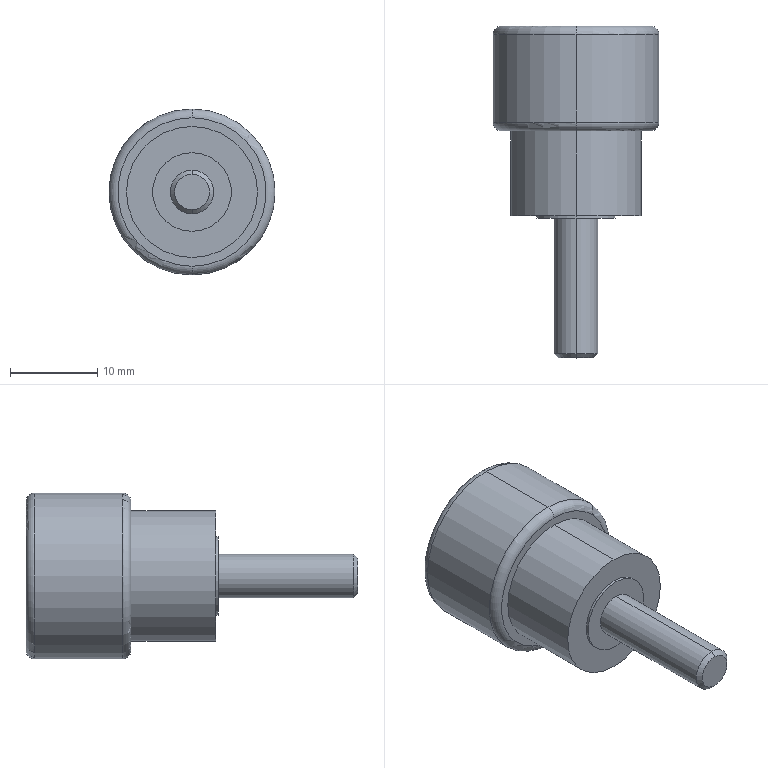Part | STEP file | Guide wheel mechanism revised.sldasm-Part-44 | 1 solid | 22 faces | box 19 x 38 x 19 mm | volume 5322 mm3 | cylinder 10 | plane 6 | torus 4 | cone 2 | commonest cylinder face diameters 5 x2 9 x2 15 x2 16 x2 19 x2
STEP:
#1=CARTESIAN_POINT('',(0.,22.,8.5));
#2=VERTEX_POINT('',#1);
#3=CARTESIAN_POINT('',(0.,22.,-8.5));
#4=VERTEX_POINT('',#3);
#5=CARTESIAN_POINT('',(0.,22.,0.));
#6=DIRECTION('',(0.,1.,0.));
#7=DIRECTION('',(0.,0.,-1.));
#8=AXIS2_PLACEMENT_3D('',#5,#6,#7);
#9=CIRCLE('',#8,8.5);
#10=EDGE_CURVE('',#2,#4,#9,.T.);
#11=ORIENTED_EDGE('',*,*,#10,.F.);
#12=CARTESIAN_POINT('',(0.,21.,9.5));
#13=VERTEX_POINT('',#12);
#14=CARTESIAN_POINT('',(0.,21.,8.5));
#15=DIRECTION('',(1.,0.,0.));
#16=DIRECTION('',(0.,0.,-1.));
#17=AXIS2_PLACEMENT_3D('',#14,#15,#16);
#18=CIRCLE('',#17,1.);
#19=EDGE_CURVE('',#2,#13,#18,.T.);
#20=ORIENTED_EDGE('',*,*,#19,.T.);
#21=CARTESIAN_POINT('',(0.,21.,-9.5));
#22=VERTEX_POINT('',#21);
#23=CARTESIAN_POINT('',(0.,21.,0.));
#24=DIRECTION('',(0.,-1.,0.));
#25=DIRECTION('',(0.,0.,-1.));
#26=AXIS2_PLACEMENT_3D('',#23,#24,#25);
#27=CIRCLE('',#26,9.5);
#28=EDGE_CURVE('',#22,#13,#27,.T.);
#29=ORIENTED_EDGE('',*,*,#28,.F.);
#30=CARTESIAN_POINT('',(0.,21.,-8.5));
#31=DIRECTION('',(-1.,0.,0.));
#32=DIRECTION('',(0.,0.,1.));
#33=AXIS2_PLACEMENT_3D('',#30,#31,#32);
#34=CIRCLE('',#33,1.);
#35=EDGE_CURVE('',#4,#22,#34,.T.);
#36=ORIENTED_EDGE('',*,*,#35,.F.);
#37=EDGE_LOOP('',(#11,#20,#29,#36));
#38=FACE_OUTER_BOUND('',#37,.T.);
#39=CARTESIAN_POINT('',(0.,21.,0.));
#40=DIRECTION('',(0.,-1.,0.));
#41=DIRECTION('',(0.,0.,-1.));
#42=AXIS2_PLACEMENT_3D('',#39,#40,#41);
#43=TOROIDAL_SURFACE('',#42,8.5,1.);
#44=ADVANCED_FACE('',(#38),#43,.T.);
#45=CARTESIAN_POINT('',(0.,10.,-8.5));
#46=VERTEX_POINT('',#45);
#47=CARTESIAN_POINT('',(0.,10.,8.5));
#48=VERTEX_POINT('',#47);
#49=CARTESIAN_POINT('',(0.,10.,0.));
#50=DIRECTION('',(0.,-1.,0.));
#51=DIRECTION('',(0.,0.,1.));
#52=AXIS2_PLACEMENT_3D('',#49,#50,#51);
#53=CIRCLE('',#52,8.5);
#54=EDGE_CURVE('',#46,#48,#53,.T.);
#55=ORIENTED_EDGE('',*,*,#54,.F.);
#56=CARTESIAN_POINT('',(0.,11.,-9.5));
#57=VERTEX_POINT('',#56);
#58=CARTESIAN_POINT('',(0.,11.,-8.5));
#59=DIRECTION('',(1.,0.,0.));
#60=DIRECTION('',(0.,0.,-1.));
#61=AXIS2_PLACEMENT_3D('',#58,#59,#60);
#62=CIRCLE('',#61,1.);
#63=EDGE_CURVE('',#46,#57,#62,.T.);
#64=ORIENTED_EDGE('',*,*,#63,.T.);
#65=CARTESIAN_POINT('',(0.,11.,9.5));
#66=VERTEX_POINT('',#65);
#67=CARTESIAN_POINT('',(0.,11.,0.));
#68=DIRECTION('',(0.,1.,0.));
#69=DIRECTION('',(0.,0.,1.));
#70=AXIS2_PLACEMENT_3D('',#67,#68,#69);
#71=CIRCLE('',#70,9.5);
#72=EDGE_CURVE('',#66,#57,#71,.T.);
#73=ORIENTED_EDGE('',*,*,#72,.F.);
#74=CARTESIAN_POINT('',(0.,11.,8.5));
#75=DIRECTION('',(-1.,0.,0.));
#76=DIRECTION('',(0.,0.,1.));
#77=AXIS2_PLACEMENT_3D('',#74,#75,#76);
#78=CIRCLE('',#77,1.);
#79=EDGE_CURVE('',#48,#66,#78,.T.);
#80=ORIENTED_EDGE('',*,*,#79,.F.);
#81=EDGE_LOOP('',(#55,#64,#73,#80));
#82=FACE_OUTER_BOUND('',#81,.T.);
#83=CARTESIAN_POINT('',(0.,11.,0.));
#84=DIRECTION('',(0.,1.,0.));
#85=DIRECTION('',(0.,0.,1.));
#86=AXIS2_PLACEMENT_3D('',#83,#84,#85);
#87=TOROIDAL_SURFACE('',#86,8.5,1.);
#88=ADVANCED_FACE('',(#82),#87,.T.);
#89=CARTESIAN_POINT('',(0.,21.5,-8.));
#90=VERTEX_POINT('',#89);
#91=CARTESIAN_POINT('',(0.,21.5,8.));
#92=VERTEX_POINT('',#91);
#93=CARTESIAN_POINT('',(0.,21.5,0.));
#94=DIRECTION('',(0.,1.,0.));
#95=DIRECTION('',(0.,0.,1.));
#96=AXIS2_PLACEMENT_3D('',#93,#94,#95);
#97=CIRCLE('',#96,8.);
#98=EDGE_CURVE('',#90,#92,#97,.T.);
#99=ORIENTED_EDGE('',*,*,#98,.F.);
#100=CARTESIAN_POINT('',(0.,22.,-8.));
#101=VERTEX_POINT('',#100);
#102=CARTESIAN_POINT('',(0.,-16.,-8.));
#103=DIRECTION('',(0.,1.,0.));
#104=VECTOR('',#103,1000.);
#105=LINE('',#102,#104);
#106=EDGE_CURVE('',#90,#101,#105,.T.);
#107=ORIENTED_EDGE('',*,*,#106,.T.);
#108=CARTESIAN_POINT('',(0.,22.,8.));
#109=VERTEX_POINT('',#108);
#110=CARTESIAN_POINT('',(0.,22.,0.));
#111=DIRECTION('',(0.,1.,0.));
#112=DIRECTION('',(0.,0.,1.));
#113=AXIS2_PLACEMENT_3D('',#110,#111,#112);
#114=CIRCLE('',#113,8.);
#115=EDGE_CURVE('',#101,#109,#114,.T.);
#116=ORIENTED_EDGE('',*,*,#115,.T.);
#117=CARTESIAN_POINT('',(0.,-16.,8.));
#118=DIRECTION('',(0.,1.,0.));
#119=VECTOR('',#118,1000.);
#120=LINE('',#117,#119);
#121=EDGE_CURVE('',#92,#109,#120,.T.);
#122=ORIENTED_EDGE('',*,*,#121,.F.);
#123=EDGE_LOOP('',(#99,#107,#116,#122));
#124=FACE_OUTER_BOUND('',#123,.T.);
#125=CARTESIAN_POINT('',(0.,-16.,0.));
#126=DIRECTION('',(0.,1.,0.));
#127=DIRECTION('',(0.,0.,1.));
#128=AXIS2_PLACEMENT_3D('',#125,#126,#127);
#129=CYLINDRICAL_SURFACE('',#128,8.);
#130=ADVANCED_FACE('',(#124),#129,.F.);
#131=ORIENTED_EDGE('',*,*,#72,.T.);
#132=CARTESIAN_POINT('',(0.,-16.,-9.5));
#133=DIRECTION('',(0.,1.,0.));
#134=VECTOR('',#133,1000.);
#135=LINE('',#132,#134);
#136=EDGE_CURVE('',#57,#22,#135,.T.);
#137=ORIENTED_EDGE('',*,*,#136,.T.);
#138=ORIENTED_EDGE('',*,*,#28,.T.);
#139=CARTESIAN_POINT('',(0.,-16.,9.5));
#140=DIRECTION('',(0.,1.,0.));
#141=VECTOR('',#140,1000.);
#142=LINE('',#139,#141);
#143=EDGE_CURVE('',#66,#13,#142,.T.);
#144=ORIENTED_EDGE('',*,*,#143,.F.);
#145=EDGE_LOOP('',(#131,#137,#138,#144));
#146=FACE_OUTER_BOUND('',#145,.T.);
#147=CARTESIAN_POINT('',(0.,-16.,0.));
#148=DIRECTION('',(0.,1.,0.));
#149=DIRECTION('',(0.,0.,1.));
#150=AXIS2_PLACEMENT_3D('',#147,#148,#149);
#151=CYLINDRICAL_SURFACE('',#150,9.5);
#152=ADVANCED_FACE('',(#146),#151,.T.);
#153=CARTESIAN_POINT('',(0.,-16.,2.01));
#154=VERTEX_POINT('',#153);
#155=CARTESIAN_POINT('',(0.,-16.,-2.01));
#156=VERTEX_POINT('',#155);
#157=CARTESIAN_POINT('',(0.,-16.,0.));
#158=DIRECTION('',(0.,1.,0.));
#159=DIRECTION('',(0.,0.,1.));
#160=AXIS2_PLACEMENT_3D('',#157,#158,#159);
#161=CIRCLE('',#160,2.01);
#162=EDGE_CURVE('',#154,#156,#161,.T.);
#163=ORIENTED_EDGE('',*,*,#162,.T.);
#164=CARTESIAN_POINT('',(0.,-15.51,-2.5));
#165=VERTEX_POINT('',#164);
#166=CARTESIAN_POINT('',(0.,-16.,-2.01));
#167=DIRECTION('',(0.,0.7071,-0.7071));
#168=VECTOR('',#167,1000.);
#169=LINE('',#166,#168);
#170=EDGE_CURVE('',#156,#165,#169,.T.);
#171=ORIENTED_EDGE('',*,*,#170,.T.);
#172=CARTESIAN_POINT('',(0.,-15.51,2.5));
#173=VERTEX_POINT('',#172);
#174=CARTESIAN_POINT('',(0.,-15.51,0.));
#175=DIRECTION('',(0.,1.,0.));
#176=DIRECTION('',(0.,0.,1.));
#177=AXIS2_PLACEMENT_3D('',#174,#175,#176);
#178=CIRCLE('',#177,2.5);
#179=EDGE_CURVE('',#173,#165,#178,.T.);
#180=ORIENTED_EDGE('',*,*,#179,.F.);
#181=CARTESIAN_POINT('',(0.,-16.,2.01));
#182=DIRECTION('',(0.,0.7071,0.7071));
#183=VECTOR('',#182,1000.);
#184=LINE('',#181,#183);
#185=EDGE_CURVE('',#154,#173,#184,.T.);
#186=ORIENTED_EDGE('',*,*,#185,.F.);
#187=EDGE_LOOP('',(#163,#171,#180,#186));
#188=FACE_OUTER_BOUND('',#187,.T.);
#189=CARTESIAN_POINT('',(0.,-16.,0.));
#190=DIRECTION('',(0.,1.,0.));
#191=DIRECTION('',(0.,0.,1.));
#192=AXIS2_PLACEMENT_3D('',#189,#190,#191);
#193=CONICAL_SURFACE('',#192,2.01,0.7854);
#194=ADVANCED_FACE('',(#188),#193,.T.);
#195=ORIENTED_EDGE('',*,*,#179,.T.);
#196=CARTESIAN_POINT('',(0.,0.,-2.5));
#197=VERTEX_POINT('',#196);
#198=CARTESIAN_POINT('',(0.,-16.,-2.5));
#199=DIRECTION('',(0.,1.,0.));
#200=VECTOR('',#199,1000.);
#201=LINE('',#198,#200);
#202=EDGE_CURVE('',#165,#197,#201,.T.);
#203=ORIENTED_EDGE('',*,*,#202,.T.);
#204=CARTESIAN_POINT('',(0.,0.,2.5));
#205=VERTEX_POINT('',#204);
#206=CARTESIAN_POINT('',(0.,0.,0.));
#207=DIRECTION('',(0.,1.,0.));
#208=DIRECTION('',(0.,0.,1.));
#209=AXIS2_PLACEMENT_3D('',#206,#207,#208);
#210=CIRCLE('',#209,2.5);
#211=EDGE_CURVE('',#205,#197,#210,.T.);
#212=ORIENTED_EDGE('',*,*,#211,.F.);
#213=CARTESIAN_POINT('',(0.,-16.,2.5));
#214=DIRECTION('',(0.,1.,0.));
#215=VECTOR('',#214,1000.);
#216=LINE('',#213,#215);
#217=EDGE_CURVE('',#173,#205,#216,.T.);
#218=ORIENTED_EDGE('',*,*,#217,.F.);
#219=EDGE_LOOP('',(#195,#203,#212,#218));
#220=FACE_OUTER_BOUND('',#219,.T.);
#221=CARTESIAN_POINT('',(0.,-16.,0.));
#222=DIRECTION('',(0.,1.,0.));
#223=DIRECTION('',(0.,0.,1.));
#224=AXIS2_PLACEMENT_3D('',#221,#222,#223);
#225=CYLINDRICAL_SURFACE('',#224,2.5);
#226=ADVANCED_FACE('',(#220),#225,.T.);
#227=CARTESIAN_POINT('',(0.,0.,4.5));
#228=VERTEX_POINT('',#227);
#229=CARTESIAN_POINT('',(0.,0.,-4.5));
#230=VERTEX_POINT('',#229);
#231=CARTESIAN_POINT('',(0.,0.,0.));
#232=DIRECTION('',(0.,1.,0.));
#233=DIRECTION('',(0.,0.,1.));
#234=AXIS2_PLACEMENT_3D('',#231,#232,#233);
#235=CIRCLE('',#234,4.5);
#236=EDGE_CURVE('',#228,#230,#235,.T.);
#237=ORIENTED_EDGE('',*,*,#236,.T.);
#238=CARTESIAN_POINT('',(0.,0.3,-4.5));
#239=VERTEX_POINT('',#238);
#240=CARTESIAN_POINT('',(0.,-16.,-4.5));
#241=DIRECTION('',(0.,1.,0.));
#242=VECTOR('',#241,1000.);
#243=LINE('',#240,#242);
#244=EDGE_CURVE('',#230,#239,#243,.T.);
#245=ORIENTED_EDGE('',*,*,#244,.T.);
#246=CARTESIAN_POINT('',(0.,0.3,4.5));
#247=VERTEX_POINT('',#246);
#248=CARTESIAN_POINT('',(0.,0.3,0.));
#249=DIRECTION('',(0.,1.,0.));
#250=DIRECTION('',(0.,0.,1.));
#251=AXIS2_PLACEMENT_3D('',#248,#249,#250);
#252=CIRCLE('',#251,4.5);
#253=EDGE_CURVE('',#247,#239,#252,.T.);
#254=ORIENTED_EDGE('',*,*,#253,.F.);
#255=CARTESIAN_POINT('',(0.,-16.,4.5));
#256=DIRECTION('',(0.,1.,0.));
#257=VECTOR('',#256,1000.);
#258=LINE('',#255,#257);
#259=EDGE_CURVE('',#228,#247,#258,.T.);
#260=ORIENTED_EDGE('',*,*,#259,.F.);
#261=EDGE_LOOP('',(#237,#245,#254,#260));
#262=FACE_OUTER_BOUND('',#261,.T.);
#263=CARTESIAN_POINT('',(0.,-16.,0.));
#264=DIRECTION('',(0.,1.,0.));
#265=DIRECTION('',(0.,0.,1.));
#266=AXIS2_PLACEMENT_3D('',#263,#264,#265);
#267=CYLINDRICAL_SURFACE('',#266,4.5);
#268=ADVANCED_FACE('',(#262),#267,.T.);
#269=CARTESIAN_POINT('',(0.,0.3,7.5));
#270=VERTEX_POINT('',#269);
#271=CARTESIAN_POINT('',(0.,0.3,-7.5));
#272=VERTEX_POINT('',#271);
#273=CARTESIAN_POINT('',(0.,0.3,0.));
#274=DIRECTION('',(0.,1.,0.));
#275=DIRECTION('',(0.,0.,1.));
#276=AXIS2_PLACEMENT_3D('',#273,#274,#275);
#277=CIRCLE('',#276,7.5);
#278=EDGE_CURVE('',#270,#272,#277,.T.);
#279=ORIENTED_EDGE('',*,*,#278,.T.);
#280=CARTESIAN_POINT('',(0.,10.,-7.5));
#281=VERTEX_POINT('',#280);
#282=CARTESIAN_POINT('',(0.,-16.,-7.5));
#283=DIRECTION('',(0.,1.,0.));
#284=VECTOR('',#283,1000.);
#285=LINE('',#282,#284);
#286=EDGE_CURVE('',#272,#281,#285,.T.);
#287=ORIENTED_EDGE('',*,*,#286,.T.);
#288=CARTESIAN_POINT('',(0.,10.,7.5));
#289=VERTEX_POINT('',#288);
#290=CARTESIAN_POINT('',(0.,10.,0.));
#291=DIRECTION('',(0.,1.,0.));
#292=DIRECTION('',(0.,0.,1.));
#293=AXIS2_PLACEMENT_3D('',#290,#291,#292);
#294=CIRCLE('',#293,7.5);
#295=EDGE_CURVE('',#289,#281,#294,.T.);
#296=ORIENTED_EDGE('',*,*,#295,.F.);
#297=CARTESIAN_POINT('',(0.,-16.,7.5));
#298=DIRECTION('',(0.,1.,0.));
#299=VECTOR('',#298,1000.);
#300=LINE('',#297,#299);
#301=EDGE_CURVE('',#270,#289,#300,.T.);
#302=ORIENTED_EDGE('',*,*,#301,.F.);
#303=EDGE_LOOP('',(#279,#287,#296,#302));
#304=FACE_OUTER_BOUND('',#303,.T.);
#305=CARTESIAN_POINT('',(0.,-16.,0.));
#306=DIRECTION('',(0.,1.,0.));
#307=DIRECTION('',(0.,0.,1.));
#308=AXIS2_PLACEMENT_3D('',#305,#306,#307);
#309=CYLINDRICAL_SURFACE('',#308,7.5);
#310=ADVANCED_FACE('',(#304),#309,.T.);
#311=CARTESIAN_POINT('',(0.,10.,0.));
#312=DIRECTION('',(0.,-1.,0.));
#313=DIRECTION('',(0.,0.,1.));
#314=AXIS2_PLACEMENT_3D('',#311,#312,#313);
#315=CIRCLE('',#314,8.5);
#316=EDGE_CURVE('',#48,#46,#315,.T.);
#317=ORIENTED_EDGE('',*,*,#316,.T.);
#318=ORIENTED_EDGE('',*,*,#54,.T.);
#319=EDGE_LOOP('',(#317,#318));
#320=FACE_OUTER_BOUND('',#319,.T.);
#321=ORIENTED_EDGE('',*,*,#295,.T.);
#322=CARTESIAN_POINT('',(0.,10.,0.));
#323=DIRECTION('',(0.,1.,0.));
#324=DIRECTION('',(0.,0.,1.));
#325=AXIS2_PLACEMENT_3D('',#322,#323,#324);
#326=CIRCLE('',#325,7.5);
#327=EDGE_CURVE('',#281,#289,#326,.T.);
#328=ORIENTED_EDGE('',*,*,#327,.T.);
#329=EDGE_LOOP('',(#321,#328));
#330=FACE_BOUND('',#329,.T.);
#331=CARTESIAN_POINT('',(15.5,10.,0.));
#332=DIRECTION('',(0.,1.,0.));
#333=DIRECTION('',(0.,0.,1.));
#334=AXIS2_PLACEMENT_3D('',#331,#332,#333);
#335=PLANE('',#334);
#336=ADVANCED_FACE('',(#320,#330),#335,.F.);
#337=ORIENTED_EDGE('',*,*,#286,.F.);
#338=CARTESIAN_POINT('',(0.,0.3,0.));
#339=DIRECTION('',(0.,1.,0.));
#340=DIRECTION('',(0.,0.,1.));
#341=AXIS2_PLACEMENT_3D('',#338,#339,#340);
#342=CIRCLE('',#341,7.5);
#343=EDGE_CURVE('',#272,#270,#342,.T.);
#344=ORIENTED_EDGE('',*,*,#343,.T.);
#345=ORIENTED_EDGE('',*,*,#301,.T.);
#346=ORIENTED_EDGE('',*,*,#327,.F.);
#347=EDGE_LOOP('',(#337,#344,#345,#346));
#348=FACE_OUTER_BOUND('',#347,.T.);
#349=CARTESIAN_POINT('',(0.,-16.,0.));
#350=DIRECTION('',(0.,1.,0.));
#351=DIRECTION('',(0.,0.,1.));
#352=AXIS2_PLACEMENT_3D('',#349,#350,#351);
#353=CYLINDRICAL_SURFACE('',#352,7.5);
#354=ADVANCED_FACE('',(#348),#353,.T.);
#355=ORIENTED_EDGE('',*,*,#278,.F.);
#356=ORIENTED_EDGE('',*,*,#343,.F.);
#357=EDGE_LOOP('',(#355,#356));
#358=FACE_OUTER_BOUND('',#357,.T.);
#359=ORIENTED_EDGE('',*,*,#253,.T.);
#360=CARTESIAN_POINT('',(0.,0.3,0.));
#361=DIRECTION('',(0.,1.,0.));
#362=DIRECTION('',(0.,0.,1.));
#363=AXIS2_PLACEMENT_3D('',#360,#361,#362);
#364=CIRCLE('',#363,4.5);
#365=EDGE_CURVE('',#239,#247,#364,.T.);
#366=ORIENTED_EDGE('',*,*,#365,.T.);
#367=EDGE_LOOP('',(#359,#366));
#368=FACE_BOUND('',#367,.T.);
#369=CARTESIAN_POINT('',(7.5,0.3,0.));
#370=DIRECTION('',(0.,1.,0.));
#371=DIRECTION('',(0.,0.,1.));
#372=AXIS2_PLACEMENT_3D('',#369,#370,#371);
#373=PLANE('',#372);
#374=ADVANCED_FACE('',(#358,#368),#373,.F.);
#375=ORIENTED_EDGE('',*,*,#244,.F.);
#376=CARTESIAN_POINT('',(0.,0.,0.));
#377=DIRECTION('',(0.,1.,0.));
#378=DIRECTION('',(0.,0.,1.));
#379=AXIS2_PLACEMENT_3D('',#376,#377,#378);
#380=CIRCLE('',#379,4.5);
#381=EDGE_CURVE('',#230,#228,#380,.T.);
#382=ORIENTED_EDGE('',*,*,#381,.T.);
#383=ORIENTED_EDGE('',*,*,#259,.T.);
#384=ORIENTED_EDGE('',*,*,#365,.F.);
#385=EDGE_LOOP('',(#375,#382,#383,#384));
#386=FACE_OUTER_BOUND('',#385,.T.);
#387=CARTESIAN_POINT('',(0.,-16.,0.));
#388=DIRECTION('',(0.,1.,0.));
#389=DIRECTION('',(0.,0.,1.));
#390=AXIS2_PLACEMENT_3D('',#387,#388,#389);
#391=CYLINDRICAL_SURFACE('',#390,4.5);
#392=ADVANCED_FACE('',(#386),#391,.T.);
#393=ORIENTED_EDGE('',*,*,#236,.F.);
#394=ORIENTED_EDGE('',*,*,#381,.F.);
#395=EDGE_LOOP('',(#393,#394));
#396=FACE_OUTER_BOUND('',#395,.T.);
#397=ORIENTED_EDGE('',*,*,#211,.T.);
#398=CARTESIAN_POINT('',(0.,0.,0.));
#399=DIRECTION('',(0.,1.,0.));
#400=DIRECTION('',(0.,0.,1.));
#401=AXIS2_PLACEMENT_3D('',#398,#399,#400);
#402=CIRCLE('',#401,2.5);
#403=EDGE_CURVE('',#197,#205,#402,.T.);
#404=ORIENTED_EDGE('',*,*,#403,.T.);
#405=EDGE_LOOP('',(#397,#404));
#406=FACE_BOUND('',#405,.T.);
#407=CARTESIAN_POINT('',(4.5,0.,0.));
#408=DIRECTION('',(0.,1.,0.));
#409=DIRECTION('',(0.,0.,1.));
#410=AXIS2_PLACEMENT_3D('',#407,#408,#409);
#411=PLANE('',#410);
#412=ADVANCED_FACE('',(#396,#406),#411,.F.);
#413=ORIENTED_EDGE('',*,*,#202,.F.);
#414=CARTESIAN_POINT('',(0.,-15.51,0.));
#415=DIRECTION('',(0.,1.,0.));
#416=DIRECTION('',(0.,0.,1.));
#417=AXIS2_PLACEMENT_3D('',#414,#415,#416);
#418=CIRCLE('',#417,2.5);
#419=EDGE_CURVE('',#165,#173,#418,.T.);
#420=ORIENTED_EDGE('',*,*,#419,.T.);
#421=ORIENTED_EDGE('',*,*,#217,.T.);
#422=ORIENTED_EDGE('',*,*,#403,.F.);
#423=EDGE_LOOP('',(#413,#420,#421,#422));
#424=FACE_OUTER_BOUND('',#423,.T.);
#425=CARTESIAN_POINT('',(0.,-16.,0.));
#426=DIRECTION('',(0.,1.,0.));
#427=DIRECTION('',(0.,0.,1.));
#428=AXIS2_PLACEMENT_3D('',#425,#426,#427);
#429=CYLINDRICAL_SURFACE('',#428,2.5);
#430=ADVANCED_FACE('',(#424),#429,.T.);
#431=ORIENTED_EDGE('',*,*,#170,.F.);
#432=CARTESIAN_POINT('',(0.,-16.,0.));
#433=DIRECTION('',(0.,1.,0.));
#434=DIRECTION('',(0.,0.,1.));
#435=AXIS2_PLACEMENT_3D('',#432,#433,#434);
#436=CIRCLE('',#435,2.01);
#437=EDGE_CURVE('',#156,#154,#436,.T.);
#438=ORIENTED_EDGE('',*,*,#437,.T.);
#439=ORIENTED_EDGE('',*,*,#185,.T.);
#440=ORIENTED_EDGE('',*,*,#419,.F.);
#441=EDGE_LOOP('',(#431,#438,#439,#440));
#442=FACE_OUTER_BOUND('',#441,.T.);
#443=CARTESIAN_POINT('',(0.,-16.,0.));
#444=DIRECTION('',(0.,1.,0.));
#445=DIRECTION('',(0.,0.,1.));
#446=AXIS2_PLACEMENT_3D('',#443,#444,#445);
#447=CONICAL_SURFACE('',#446,2.01,0.7854);
#448=ADVANCED_FACE('',(#442),#447,.T.);
#449=ORIENTED_EDGE('',*,*,#162,.F.);
#450=ORIENTED_EDGE('',*,*,#437,.F.);
#451=EDGE_LOOP('',(#449,#450));
#452=FACE_OUTER_BOUND('',#451,.T.);
#453=CARTESIAN_POINT('',(2.01,-16.,0.));
#454=DIRECTION('',(0.,1.,0.));
#455=DIRECTION('',(0.,0.,1.));
#456=AXIS2_PLACEMENT_3D('',#453,#454,#455);
#457=PLANE('',#456);
#458=ADVANCED_FACE('',(#452),#457,.F.);
#459=ORIENTED_EDGE('',*,*,#136,.F.);
#460=CARTESIAN_POINT('',(0.,11.,0.));
#461=DIRECTION('',(0.,1.,0.));
#462=DIRECTION('',(0.,0.,1.));
#463=AXIS2_PLACEMENT_3D('',#460,#461,#462);
#464=CIRCLE('',#463,9.5);
#465=EDGE_CURVE('',#57,#66,#464,.T.);
#466=ORIENTED_EDGE('',*,*,#465,.T.);
#467=ORIENTED_EDGE('',*,*,#143,.T.);
#468=CARTESIAN_POINT('',(0.,21.,0.));
#469=DIRECTION('',(0.,-1.,0.));
#470=DIRECTION('',(0.,0.,-1.));
#471=AXIS2_PLACEMENT_3D('',#468,#469,#470);
#472=CIRCLE('',#471,9.5);
#473=EDGE_CURVE('',#13,#22,#472,.T.);
#474=ORIENTED_EDGE('',*,*,#473,.T.);
#475=EDGE_LOOP('',(#459,#466,#467,#474));
#476=FACE_OUTER_BOUND('',#475,.T.);
#477=CARTESIAN_POINT('',(0.,-16.,0.));
#478=DIRECTION('',(0.,1.,0.));
#479=DIRECTION('',(0.,0.,1.));
#480=AXIS2_PLACEMENT_3D('',#477,#478,#479);
#481=CYLINDRICAL_SURFACE('',#480,9.5);
#482=ADVANCED_FACE('',(#476),#481,.T.);
#483=CARTESIAN_POINT('',(0.,21.5,0.));
#484=DIRECTION('',(0.,1.,0.));
#485=DIRECTION('',(0.,0.,1.));
#486=AXIS2_PLACEMENT_3D('',#483,#484,#485);
#487=CIRCLE('',#486,8.);
#488=EDGE_CURVE('',#92,#90,#487,.T.);
#489=ORIENTED_EDGE('',*,*,#488,.T.);
#490=ORIENTED_EDGE('',*,*,#98,.T.);
#491=EDGE_LOOP('',(#489,#490));
#492=FACE_OUTER_BOUND('',#491,.T.);
#493=CARTESIAN_POINT('',(0.,21.5,0.));
#494=DIRECTION('',(0.,-1.,0.));
#495=DIRECTION('',(0.,0.,-1.));
#496=AXIS2_PLACEMENT_3D('',#493,#494,#495);
#497=PLANE('',#496);
#498=ADVANCED_FACE('',(#492),#497,.F.);
#499=ORIENTED_EDGE('',*,*,#106,.F.);
#500=ORIENTED_EDGE('',*,*,#488,.F.);
#501=ORIENTED_EDGE('',*,*,#121,.T.);
#502=CARTESIAN_POINT('',(0.,22.,0.));
#503=DIRECTION('',(0.,1.,0.));
#504=DIRECTION('',(0.,0.,1.));
#505=AXIS2_PLACEMENT_3D('',#502,#503,#504);
#506=CIRCLE('',#505,8.);
#507=EDGE_CURVE('',#109,#101,#506,.T.);
#508=ORIENTED_EDGE('',*,*,#507,.T.);
#509=EDGE_LOOP('',(#499,#500,#501,#508));
#510=FACE_OUTER_BOUND('',#509,.T.);
#511=CARTESIAN_POINT('',(0.,-16.,0.));
#512=DIRECTION('',(0.,1.,0.));
#513=DIRECTION('',(0.,0.,1.));
#514=AXIS2_PLACEMENT_3D('',#511,#512,#513);
#515=CYLINDRICAL_SURFACE('',#514,8.);
#516=ADVANCED_FACE('',(#510),#515,.F.);
#517=CARTESIAN_POINT('',(0.,22.,0.));
#518=DIRECTION('',(0.,1.,0.));
#519=DIRECTION('',(0.,0.,-1.));
#520=AXIS2_PLACEMENT_3D('',#517,#518,#519);
#521=CIRCLE('',#520,8.5);
#522=EDGE_CURVE('',#4,#2,#521,.T.);
#523=ORIENTED_EDGE('',*,*,#522,.T.);
#524=ORIENTED_EDGE('',*,*,#10,.T.);
#525=EDGE_LOOP('',(#523,#524));
#526=FACE_OUTER_BOUND('',#525,.T.);
#527=ORIENTED_EDGE('',*,*,#507,.F.);
#528=ORIENTED_EDGE('',*,*,#115,.F.);
#529=EDGE_LOOP('',(#527,#528));
#530=FACE_BOUND('',#529,.T.);
#531=CARTESIAN_POINT('',(8.,22.,0.));
#532=DIRECTION('',(0.,-1.,0.));
#533=DIRECTION('',(0.,0.,-1.));
#534=AXIS2_PLACEMENT_3D('',#531,#532,#533);
#535=PLANE('',#534);
#536=ADVANCED_FACE('',(#526,#530),#535,.F.);
#537=ORIENTED_EDGE('',*,*,#63,.F.);
#538=ORIENTED_EDGE('',*,*,#316,.F.);
#539=ORIENTED_EDGE('',*,*,#79,.T.);
#540=ORIENTED_EDGE('',*,*,#465,.F.);
#541=EDGE_LOOP('',(#537,#538,#539,#540));
#542=FACE_OUTER_BOUND('',#541,.T.);
#543=CARTESIAN_POINT('',(0.,11.,0.));
#544=DIRECTION('',(0.,1.,0.));
#545=DIRECTION('',(0.,0.,1.));
#546=AXIS2_PLACEMENT_3D('',#543,#544,#545);
#547=TOROIDAL_SURFACE('',#546,8.5,1.);
#548=ADVANCED_FACE('',(#542),#547,.T.);
#549=ORIENTED_EDGE('',*,*,#19,.F.);
#550=ORIENTED_EDGE('',*,*,#522,.F.);
#551=ORIENTED_EDGE('',*,*,#35,.T.);
#552=ORIENTED_EDGE('',*,*,#473,.F.);
#553=EDGE_LOOP('',(#549,#550,#551,#552));
#554=FACE_OUTER_BOUND('',#553,.T.);
#555=CARTESIAN_POINT('',(0.,21.,0.));
#556=DIRECTION('',(0.,-1.,0.));
#557=DIRECTION('',(0.,0.,-1.));
#558=AXIS2_PLACEMENT_3D('',#555,#556,#557);
#559=TOROIDAL_SURFACE('',#558,8.5,1.);
#560=ADVANCED_FACE('',(#554),#559,.T.);
#561=CLOSED_SHELL('',(#44,#88,#130,#152,#194,#226,#268,#310,#336,#354,#374,#392,#412,#430,#448,#458,#482,#498,#516,#536,#548,#560));
#562=MANIFOLD_SOLID_BREP('',#561);
#563=CARTESIAN_POINT('',(0.,0.,0.));
#564=DIRECTION('',(0.,0.,1.));
#565=DIRECTION('',(1.,0.,0.));
#566=AXIS2_PLACEMENT_3D('',#563,#564,#565);
#567=(LENGTH_UNIT()NAMED_UNIT(*)SI_UNIT(.MILLI.,.METRE.));
#568=UNCERTAINTY_MEASURE_WITH_UNIT(LENGTH_MEASURE(0.00001),#567,'','');
#569=(NAMED_UNIT(*)PLANE_ANGLE_UNIT()SI_UNIT($,.RADIAN.));
#570=(NAMED_UNIT(*)SI_UNIT($,.STERADIAN.)SOLID_ANGLE_UNIT());
#571=(GEOMETRIC_REPRESENTATION_CONTEXT(3)GLOBAL_UNCERTAINTY_ASSIGNED_CONTEXT((#568))GLOBAL_UNIT_ASSIGNED_CONTEXT((#567,#569,#570))REPRESENTATION_CONTEXT('',''));
#572=ADVANCED_BREP_SHAPE_REPRESENTATION('',(#562,#566),#571);